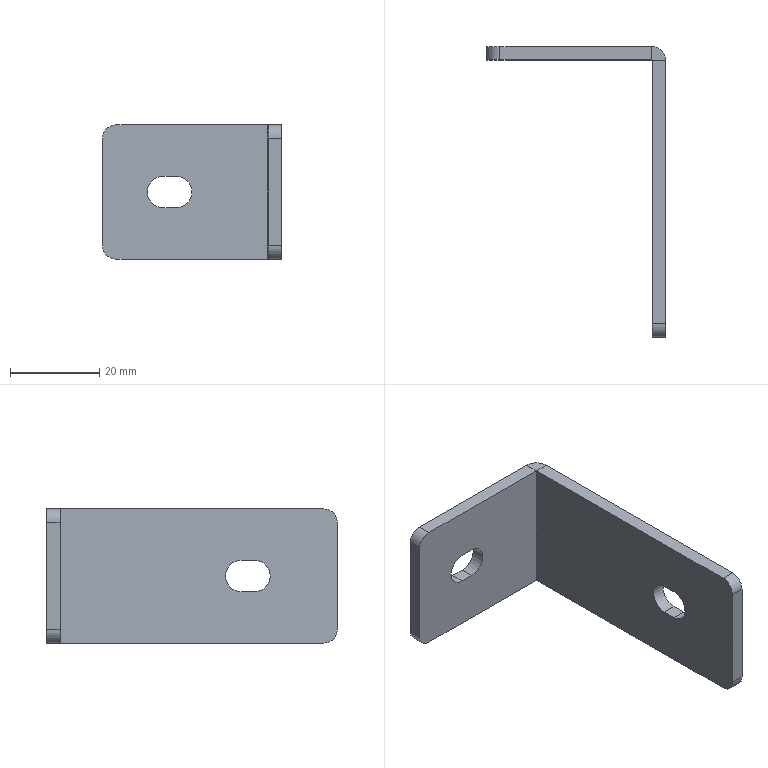Part | STEP file | Kanban profile mounting bracket | 1 solid | 27 faces | box 40 x 65 x 30 mm | volume 8738 mm3 | plane 16 | cylinder 11 | commonest cylinder face diameters 7 x5 6 x4 0.2 x1 6.2 x1